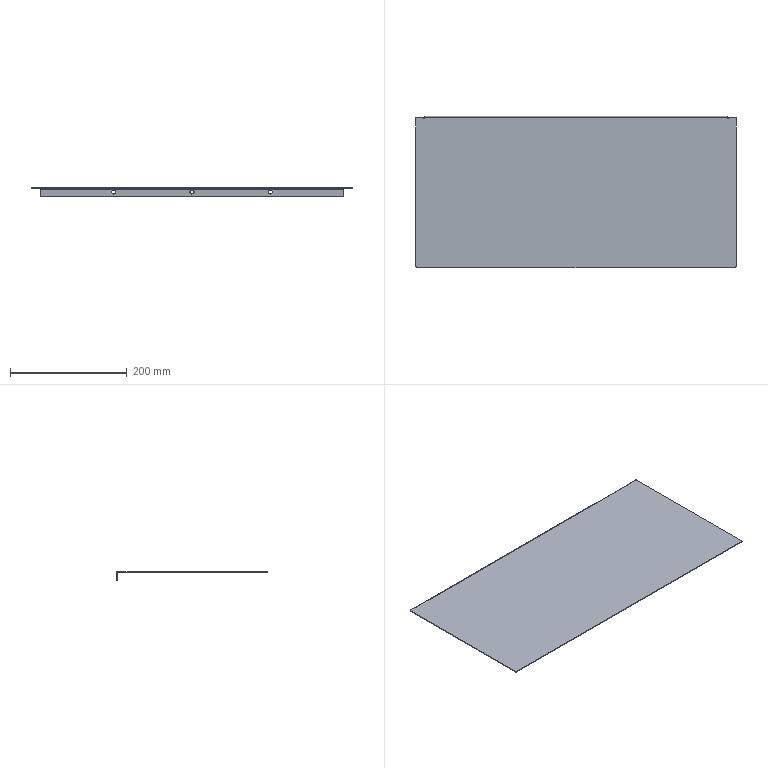Part | SolidWorks | features EdgeFlange 1, FlatPattern 1, ICE 1, SMBaseFlange 1, SheetMetal 1 | 1 solid | 32 faces | box 547.6 x 258.8 x 15 mm | volume 177930 mm3 | plane 20 | cylinder 12 | commonest cylinder face diameters 7 x6 3 x5 5.4 x1
STEP:
#1=CARTESIAN_POINT('',(133.75,258.8,-11.));
#2=VERTEX_POINT('',#1);
#3=CARTESIAN_POINT('',(133.75,258.8,-4.));
#4=VERTEX_POINT('',#3);
#5=CARTESIAN_POINT('',(133.75,258.8,-7.5));
#6=DIRECTION('',(0.,1.,0.));
#7=DIRECTION('',(0.,0.,1.));
#8=AXIS2_PLACEMENT_3D('',#5,#6,#7);
#9=CIRCLE('',#8,3.5);
#10=EDGE_CURVE('',#2,#4,#9,.T.);
#11=ORIENTED_EDGE('',*,*,#10,.F.);
#12=CARTESIAN_POINT('',(133.75,260.,-11.));
#13=VERTEX_POINT('',#12);
#14=CARTESIAN_POINT('',(133.75,250.,-11.));
#15=DIRECTION('',(0.,1.,0.));
#16=VECTOR('',#15,1000.);
#17=LINE('',#14,#16);
#18=EDGE_CURVE('',#2,#13,#17,.T.);
#19=ORIENTED_EDGE('',*,*,#18,.T.);
#20=CARTESIAN_POINT('',(133.75,260.,-4.));
#21=VERTEX_POINT('',#20);
#22=CARTESIAN_POINT('',(133.75,260.,-7.5));
#23=DIRECTION('',(0.,1.,0.));
#24=DIRECTION('',(0.,0.,1.));
#25=AXIS2_PLACEMENT_3D('',#22,#23,#24);
#26=CIRCLE('',#25,3.5);
#27=EDGE_CURVE('',#13,#21,#26,.T.);
#28=ORIENTED_EDGE('',*,*,#27,.T.);
#29=CARTESIAN_POINT('',(133.75,250.,-4.));
#30=DIRECTION('',(0.,1.,0.));
#31=VECTOR('',#30,1000.);
#32=LINE('',#29,#31);
#33=EDGE_CURVE('',#4,#21,#32,.T.);
#34=ORIENTED_EDGE('',*,*,#33,.F.);
#35=EDGE_LOOP('',(#11,#19,#28,#34));
#36=FACE_OUTER_BOUND('',#35,.T.);
#37=CARTESIAN_POINT('',(133.75,250.,-7.5));
#38=DIRECTION('',(0.,1.,0.));
#39=DIRECTION('',(0.,0.,1.));
#40=AXIS2_PLACEMENT_3D('',#37,#38,#39);
#41=CYLINDRICAL_SURFACE('',#40,3.5);
#42=ADVANCED_FACE('',(#36),#41,.F.);
#43=CARTESIAN_POINT('',(-133.75,258.8,-11.));
#44=VERTEX_POINT('',#43);
#45=CARTESIAN_POINT('',(-133.75,258.8,-4.));
#46=VERTEX_POINT('',#45);
#47=CARTESIAN_POINT('',(-133.75,258.8,-7.5));
#48=DIRECTION('',(0.,1.,0.));
#49=DIRECTION('',(0.,0.,1.));
#50=AXIS2_PLACEMENT_3D('',#47,#48,#49);
#51=CIRCLE('',#50,3.5);
#52=EDGE_CURVE('',#44,#46,#51,.T.);
#53=ORIENTED_EDGE('',*,*,#52,.F.);
#54=CARTESIAN_POINT('',(-133.75,260.,-11.));
#55=VERTEX_POINT('',#54);
#56=CARTESIAN_POINT('',(-133.75,250.,-11.));
#57=DIRECTION('',(0.,1.,0.));
#58=VECTOR('',#57,1000.);
#59=LINE('',#56,#58);
#60=EDGE_CURVE('',#44,#55,#59,.T.);
#61=ORIENTED_EDGE('',*,*,#60,.T.);
#62=CARTESIAN_POINT('',(-133.75,260.,-4.));
#63=VERTEX_POINT('',#62);
#64=CARTESIAN_POINT('',(-133.75,260.,-7.5));
#65=DIRECTION('',(0.,1.,0.));
#66=DIRECTION('',(0.,0.,1.));
#67=AXIS2_PLACEMENT_3D('',#64,#65,#66);
#68=CIRCLE('',#67,3.5);
#69=EDGE_CURVE('',#55,#63,#68,.T.);
#70=ORIENTED_EDGE('',*,*,#69,.T.);
#71=CARTESIAN_POINT('',(-133.75,250.,-4.));
#72=DIRECTION('',(0.,1.,0.));
#73=VECTOR('',#72,1000.);
#74=LINE('',#71,#73);
#75=EDGE_CURVE('',#46,#63,#74,.T.);
#76=ORIENTED_EDGE('',*,*,#75,.F.);
#77=EDGE_LOOP('',(#53,#61,#70,#76));
#78=FACE_OUTER_BOUND('',#77,.T.);
#79=CARTESIAN_POINT('',(-133.75,250.,-7.5));
#80=DIRECTION('',(0.,1.,0.));
#81=DIRECTION('',(0.,0.,1.));
#82=AXIS2_PLACEMENT_3D('',#79,#80,#81);
#83=CYLINDRICAL_SURFACE('',#82,3.5);
#84=ADVANCED_FACE('',(#78),#83,.F.);
#85=CARTESIAN_POINT('',(0.,258.8,-11.));
#86=VERTEX_POINT('',#85);
#87=CARTESIAN_POINT('',(0.,258.8,-4.));
#88=VERTEX_POINT('',#87);
#89=CARTESIAN_POINT('',(0.,258.8,-7.5));
#90=DIRECTION('',(0.,1.,0.));
#91=DIRECTION('',(0.,0.,1.));
#92=AXIS2_PLACEMENT_3D('',#89,#90,#91);
#93=CIRCLE('',#92,3.5);
#94=EDGE_CURVE('',#86,#88,#93,.T.);
#95=ORIENTED_EDGE('',*,*,#94,.F.);
#96=CARTESIAN_POINT('',(0.,260.,-11.));
#97=VERTEX_POINT('',#96);
#98=CARTESIAN_POINT('',(0.,250.,-11.));
#99=DIRECTION('',(0.,1.,0.));
#100=VECTOR('',#99,1000.);
#101=LINE('',#98,#100);
#102=EDGE_CURVE('',#86,#97,#101,.T.);
#103=ORIENTED_EDGE('',*,*,#102,.T.);
#104=CARTESIAN_POINT('',(0.,260.,-4.));
#105=VERTEX_POINT('',#104);
#106=CARTESIAN_POINT('',(0.,260.,-7.5));
#107=DIRECTION('',(0.,1.,0.));
#108=DIRECTION('',(0.,0.,1.));
#109=AXIS2_PLACEMENT_3D('',#106,#107,#108);
#110=CIRCLE('',#109,3.5);
#111=EDGE_CURVE('',#97,#105,#110,.T.);
#112=ORIENTED_EDGE('',*,*,#111,.T.);
#113=CARTESIAN_POINT('',(0.,250.,-4.));
#114=DIRECTION('',(0.,1.,0.));
#115=VECTOR('',#114,1000.);
#116=LINE('',#113,#115);
#117=EDGE_CURVE('',#88,#105,#116,.T.);
#118=ORIENTED_EDGE('',*,*,#117,.F.);
#119=EDGE_LOOP('',(#95,#103,#112,#118));
#120=FACE_OUTER_BOUND('',#119,.T.);
#121=CARTESIAN_POINT('',(0.,250.,-7.5));
#122=DIRECTION('',(0.,1.,0.));
#123=DIRECTION('',(0.,0.,1.));
#124=AXIS2_PLACEMENT_3D('',#121,#122,#123);
#125=CYLINDRICAL_SURFACE('',#124,3.5);
#126=ADVANCED_FACE('',(#120),#125,.F.);
#127=CARTESIAN_POINT('',(-260.12,258.8,0.));
#128=VERTEX_POINT('',#127);
#129=CARTESIAN_POINT('',(-272.3,258.8,0.));
#130=VERTEX_POINT('',#129);
#131=CARTESIAN_POINT('',(-272.3,258.8,0.));
#132=DIRECTION('',(-1.,0.,0.));
#133=VECTOR('',#132,1000.);
#134=LINE('',#131,#133);
#135=EDGE_CURVE('',#128,#130,#134,.T.);
#136=ORIENTED_EDGE('',*,*,#135,.F.);
#137=CARTESIAN_POINT('',(-260.12,258.8,-1.2));
#138=VERTEX_POINT('',#137);
#139=CARTESIAN_POINT('',(-260.12,258.8,-1.2));
#140=DIRECTION('',(0.,0.,-1.));
#141=VECTOR('',#140,1000.);
#142=LINE('',#139,#141);
#143=EDGE_CURVE('',#128,#138,#142,.T.);
#144=ORIENTED_EDGE('',*,*,#143,.T.);
#145=CARTESIAN_POINT('',(-272.3,258.8,-1.2));
#146=VERTEX_POINT('',#145);
#147=CARTESIAN_POINT('',(-272.3,258.8,-1.2));
#148=DIRECTION('',(-1.,0.,0.));
#149=VECTOR('',#148,1000.);
#150=LINE('',#147,#149);
#151=EDGE_CURVE('',#138,#146,#150,.T.);
#152=ORIENTED_EDGE('',*,*,#151,.T.);
#153=CARTESIAN_POINT('',(-272.3,258.8,-1.2));
#154=DIRECTION('',(0.,0.,1.));
#155=VECTOR('',#154,1000.);
#156=LINE('',#153,#155);
#157=EDGE_CURVE('',#146,#130,#156,.T.);
#158=ORIENTED_EDGE('',*,*,#157,.T.);
#159=EDGE_LOOP('',(#136,#144,#152,#158));
#160=FACE_OUTER_BOUND('',#159,.T.);
#161=CARTESIAN_POINT('',(-272.3,258.8,-1.2));
#162=DIRECTION('',(0.,1.,0.));
#163=DIRECTION('',(0.,0.,1.));
#164=AXIS2_PLACEMENT_3D('',#161,#162,#163);
#165=PLANE('',#164);
#166=ADVANCED_FACE('',(#160),#165,.T.);
#167=CARTESIAN_POINT('',(272.3,258.8,-1.2));
#168=VERTEX_POINT('',#167);
#169=CARTESIAN_POINT('',(260.12,258.8,-1.2));
#170=VERTEX_POINT('',#169);
#171=CARTESIAN_POINT('',(260.,258.8,-1.2));
#172=DIRECTION('',(-1.,0.,0.));
#173=VECTOR('',#172,1000.);
#174=LINE('',#171,#173);
#175=EDGE_CURVE('',#168,#170,#174,.T.);
#176=ORIENTED_EDGE('',*,*,#175,.T.);
#177=CARTESIAN_POINT('',(260.12,258.8,0.));
#178=VERTEX_POINT('',#177);
#179=CARTESIAN_POINT('',(260.12,258.8,-1.2));
#180=DIRECTION('',(0.,0.,1.));
#181=VECTOR('',#180,1000.);
#182=LINE('',#179,#181);
#183=EDGE_CURVE('',#170,#178,#182,.T.);
#184=ORIENTED_EDGE('',*,*,#183,.T.);
#185=CARTESIAN_POINT('',(272.3,258.8,0.));
#186=VERTEX_POINT('',#185);
#187=CARTESIAN_POINT('',(260.,258.8,0.));
#188=DIRECTION('',(-1.,0.,0.));
#189=VECTOR('',#188,1000.);
#190=LINE('',#187,#189);
#191=EDGE_CURVE('',#186,#178,#190,.T.);
#192=ORIENTED_EDGE('',*,*,#191,.F.);
#193=CARTESIAN_POINT('',(272.3,258.8,-1.2));
#194=DIRECTION('',(0.,0.,1.));
#195=VECTOR('',#194,1000.);
#196=LINE('',#193,#195);
#197=EDGE_CURVE('',#168,#186,#196,.T.);
#198=ORIENTED_EDGE('',*,*,#197,.F.);
#199=EDGE_LOOP('',(#176,#184,#192,#198));
#200=FACE_OUTER_BOUND('',#199,.T.);
#201=CARTESIAN_POINT('',(260.,258.8,-1.2));
#202=DIRECTION('',(0.,1.,0.));
#203=DIRECTION('',(0.,0.,1.));
#204=AXIS2_PLACEMENT_3D('',#201,#202,#203);
#205=PLANE('',#204);
#206=ADVANCED_FACE('',(#200),#205,.T.);
#207=CARTESIAN_POINT('',(260.12,257.18,-1.2));
#208=VERTEX_POINT('',#207);
#209=CARTESIAN_POINT('',(260.12,260.,-1.2));
#210=DIRECTION('',(0.,-1.,0.));
#211=VECTOR('',#210,1000.);
#212=LINE('',#209,#211);
#213=EDGE_CURVE('',#170,#208,#212,.T.);
#214=ORIENTED_EDGE('',*,*,#213,.F.);
#215=ORIENTED_EDGE('',*,*,#175,.F.);
#216=CARTESIAN_POINT('',(273.8,257.3,-1.2));
#217=VERTEX_POINT('',#216);
#218=CARTESIAN_POINT('',(272.3,257.3,-1.2));
#219=DIRECTION('',(0.,0.,1.));
#220=DIRECTION('',(1.,0.,0.));
#221=AXIS2_PLACEMENT_3D('',#218,#219,#220);
#222=CIRCLE('',#221,1.5);
#223=EDGE_CURVE('',#217,#168,#222,.T.);
#224=ORIENTED_EDGE('',*,*,#223,.F.);
#225=CARTESIAN_POINT('',(273.8,2.7,-1.2));
#226=VERTEX_POINT('',#225);
#227=CARTESIAN_POINT('',(273.8,257.3,-1.2));
#228=DIRECTION('',(0.,1.,0.));
#229=VECTOR('',#228,1000.);
#230=LINE('',#227,#229);
#231=EDGE_CURVE('',#226,#217,#230,.T.);
#232=ORIENTED_EDGE('',*,*,#231,.F.);
#233=CARTESIAN_POINT('',(272.3,1.2,-1.2));
#234=VERTEX_POINT('',#233);
#235=CARTESIAN_POINT('',(272.3,2.7,-1.2));
#236=DIRECTION('',(0.,0.,1.));
#237=DIRECTION('',(1.,0.,0.));
#238=AXIS2_PLACEMENT_3D('',#235,#236,#237);
#239=CIRCLE('',#238,1.5);
#240=EDGE_CURVE('',#234,#226,#239,.T.);
#241=ORIENTED_EDGE('',*,*,#240,.F.);
#242=CARTESIAN_POINT('',(-272.3,1.2,-1.2));
#243=VERTEX_POINT('',#242);
#244=CARTESIAN_POINT('',(272.3,1.2,-1.2));
#245=DIRECTION('',(1.,0.,0.));
#246=VECTOR('',#245,1000.);
#247=LINE('',#244,#246);
#248=EDGE_CURVE('',#243,#234,#247,.T.);
#249=ORIENTED_EDGE('',*,*,#248,.F.);
#250=CARTESIAN_POINT('',(-273.8,2.7,-1.2));
#251=VERTEX_POINT('',#250);
#252=CARTESIAN_POINT('',(-272.3,2.7,-1.2));
#253=DIRECTION('',(0.,0.,1.));
#254=DIRECTION('',(1.,0.,0.));
#255=AXIS2_PLACEMENT_3D('',#252,#253,#254);
#256=CIRCLE('',#255,1.5);
#257=EDGE_CURVE('',#251,#243,#256,.T.);
#258=ORIENTED_EDGE('',*,*,#257,.F.);
#259=CARTESIAN_POINT('',(-273.8,257.3,-1.2));
#260=VERTEX_POINT('',#259);
#261=CARTESIAN_POINT('',(-273.8,2.7,-1.2));
#262=DIRECTION('',(0.,-1.,0.));
#263=VECTOR('',#262,1000.);
#264=LINE('',#261,#263);
#265=EDGE_CURVE('',#260,#251,#264,.T.);
#266=ORIENTED_EDGE('',*,*,#265,.F.);
#267=CARTESIAN_POINT('',(-272.3,257.3,-1.2));
#268=DIRECTION('',(0.,0.,1.));
#269=DIRECTION('',(1.,0.,0.));
#270=AXIS2_PLACEMENT_3D('',#267,#268,#269);
#271=CIRCLE('',#270,1.5);
#272=EDGE_CURVE('',#146,#260,#271,.T.);
#273=ORIENTED_EDGE('',*,*,#272,.F.);
#274=ORIENTED_EDGE('',*,*,#151,.F.);
#275=CARTESIAN_POINT('',(-260.12,257.18,-1.2));
#276=VERTEX_POINT('',#275);
#277=CARTESIAN_POINT('',(-260.12,257.18,-1.2));
#278=DIRECTION('',(0.,1.,0.));
#279=VECTOR('',#278,1000.);
#280=LINE('',#277,#279);
#281=EDGE_CURVE('',#276,#138,#280,.T.);
#282=ORIENTED_EDGE('',*,*,#281,.F.);
#283=CARTESIAN_POINT('',(-260.,257.18,-1.2));
#284=VERTEX_POINT('',#283);
#285=CARTESIAN_POINT('',(-260.,257.18,-1.2));
#286=DIRECTION('',(-1.,0.,0.));
#287=VECTOR('',#286,1000.);
#288=LINE('',#285,#287);
#289=EDGE_CURVE('',#284,#276,#288,.T.);
#290=ORIENTED_EDGE('',*,*,#289,.F.);
#291=CARTESIAN_POINT('',(-260.,257.3,-1.2));
#292=VERTEX_POINT('',#291);
#293=CARTESIAN_POINT('',(-260.,257.3,-1.2));
#294=DIRECTION('',(0.,-1.,0.));
#295=VECTOR('',#294,1000.);
#296=LINE('',#293,#295);
#297=EDGE_CURVE('',#292,#284,#296,.T.);
#298=ORIENTED_EDGE('',*,*,#297,.F.);
#299=CARTESIAN_POINT('',(260.,257.3,-1.2));
#300=VERTEX_POINT('',#299);
#301=CARTESIAN_POINT('',(260.,257.3,-1.2));
#302=DIRECTION('',(-1.,0.,0.));
#303=VECTOR('',#302,1000.);
#304=LINE('',#301,#303);
#305=EDGE_CURVE('',#300,#292,#304,.T.);
#306=ORIENTED_EDGE('',*,*,#305,.F.);
#307=CARTESIAN_POINT('',(260.,257.18,-1.2));
#308=VERTEX_POINT('',#307);
#309=CARTESIAN_POINT('',(260.,257.18,-1.2));
#310=DIRECTION('',(0.,1.,0.));
#311=VECTOR('',#310,1000.);
#312=LINE('',#309,#311);
#313=EDGE_CURVE('',#308,#300,#312,.T.);
#314=ORIENTED_EDGE('',*,*,#313,.F.);
#315=CARTESIAN_POINT('',(260.12,257.18,-1.2));
#316=DIRECTION('',(-1.,0.,0.));
#317=VECTOR('',#316,1000.);
#318=LINE('',#315,#317);
#319=EDGE_CURVE('',#208,#308,#318,.T.);
#320=ORIENTED_EDGE('',*,*,#319,.F.);
#321=EDGE_LOOP('',(#214,#215,#224,#232,#241,#249,#258,#266,#273,#274,#282,#290,#298,#306,#314,#320));
#322=FACE_OUTER_BOUND('',#321,.T.);
#323=CARTESIAN_POINT('',(-272.3,257.3,-1.2));
#324=DIRECTION('',(0.,0.,1.));
#325=DIRECTION('',(1.,0.,0.));
#326=AXIS2_PLACEMENT_3D('',#323,#324,#325);
#327=PLANE('',#326);
#328=ADVANCED_FACE('',(#322),#327,.F.);
#329=ORIENTED_EDGE('',*,*,#191,.T.);
#330=CARTESIAN_POINT('',(260.12,257.18,0.));
#331=VERTEX_POINT('',#330);
#332=CARTESIAN_POINT('',(260.12,257.3,0.));
#333=DIRECTION('',(0.,-1.,0.));
#334=VECTOR('',#333,1000.);
#335=LINE('',#332,#334);
#336=EDGE_CURVE('',#178,#331,#335,.T.);
#337=ORIENTED_EDGE('',*,*,#336,.T.);
#338=CARTESIAN_POINT('',(260.,257.18,0.));
#339=VERTEX_POINT('',#338);
#340=CARTESIAN_POINT('',(-272.3,257.18,0.));
#341=DIRECTION('',(-1.,0.,0.));
#342=VECTOR('',#341,1000.);
#343=LINE('',#340,#342);
#344=EDGE_CURVE('',#331,#339,#343,.T.);
#345=ORIENTED_EDGE('',*,*,#344,.T.);
#346=CARTESIAN_POINT('',(260.,257.3,0.));
#347=VERTEX_POINT('',#346);
#348=CARTESIAN_POINT('',(260.,257.3,0.));
#349=DIRECTION('',(0.,1.,0.));
#350=VECTOR('',#349,1000.);
#351=LINE('',#348,#350);
#352=EDGE_CURVE('',#339,#347,#351,.T.);
#353=ORIENTED_EDGE('',*,*,#352,.T.);
#354=CARTESIAN_POINT('',(-260.,257.3,0.));
#355=VERTEX_POINT('',#354);
#356=CARTESIAN_POINT('',(260.,257.3,0.));
#357=DIRECTION('',(-1.,0.,0.));
#358=VECTOR('',#357,1000.);
#359=LINE('',#356,#358);
#360=EDGE_CURVE('',#347,#355,#359,.T.);
#361=ORIENTED_EDGE('',*,*,#360,.T.);
#362=CARTESIAN_POINT('',(-260.,257.18,0.));
#363=VERTEX_POINT('',#362);
#364=CARTESIAN_POINT('',(-260.,257.3,0.));
#365=DIRECTION('',(0.,-1.,0.));
#366=VECTOR('',#365,1000.);
#367=LINE('',#364,#366);
#368=EDGE_CURVE('',#355,#363,#367,.T.);
#369=ORIENTED_EDGE('',*,*,#368,.T.);
#370=CARTESIAN_POINT('',(-260.12,257.18,0.));
#371=VERTEX_POINT('',#370);
#372=CARTESIAN_POINT('',(-272.3,257.18,0.));
#373=DIRECTION('',(-1.,0.,0.));
#374=VECTOR('',#373,1000.);
#375=LINE('',#372,#374);
#376=EDGE_CURVE('',#363,#371,#375,.T.);
#377=ORIENTED_EDGE('',*,*,#376,.T.);
#378=CARTESIAN_POINT('',(-260.12,257.3,0.));
#379=DIRECTION('',(0.,1.,0.));
#380=VECTOR('',#379,1000.);
#381=LINE('',#378,#380);
#382=EDGE_CURVE('',#371,#128,#381,.T.);
#383=ORIENTED_EDGE('',*,*,#382,.T.);
#384=ORIENTED_EDGE('',*,*,#135,.T.);
#385=CARTESIAN_POINT('',(-273.8,257.3,0.));
#386=VERTEX_POINT('',#385);
#387=CARTESIAN_POINT('',(-272.3,257.3,0.));
#388=DIRECTION('',(0.,0.,1.));
#389=DIRECTION('',(1.,0.,0.));
#390=AXIS2_PLACEMENT_3D('',#387,#388,#389);
#391=CIRCLE('',#390,1.5);
#392=EDGE_CURVE('',#130,#386,#391,.T.);
#393=ORIENTED_EDGE('',*,*,#392,.T.);
#394=CARTESIAN_POINT('',(-273.8,2.7,0.));
#395=VERTEX_POINT('',#394);
#396=CARTESIAN_POINT('',(-273.8,2.7,0.));
#397=DIRECTION('',(0.,-1.,0.));
#398=VECTOR('',#397,1000.);
#399=LINE('',#396,#398);
#400=EDGE_CURVE('',#386,#395,#399,.T.);
#401=ORIENTED_EDGE('',*,*,#400,.T.);
#402=CARTESIAN_POINT('',(-272.3,1.2,0.));
#403=VERTEX_POINT('',#402);
#404=CARTESIAN_POINT('',(-272.3,2.7,0.));
#405=DIRECTION('',(0.,0.,1.));
#406=DIRECTION('',(1.,0.,0.));
#407=AXIS2_PLACEMENT_3D('',#404,#405,#406);
#408=CIRCLE('',#407,1.5);
#409=EDGE_CURVE('',#395,#403,#408,.T.);
#410=ORIENTED_EDGE('',*,*,#409,.T.);
#411=CARTESIAN_POINT('',(272.3,1.2,0.));
#412=VERTEX_POINT('',#411);
#413=CARTESIAN_POINT('',(272.3,1.2,0.));
#414=DIRECTION('',(1.,0.,0.));
#415=VECTOR('',#414,1000.);
#416=LINE('',#413,#415);
#417=EDGE_CURVE('',#403,#412,#416,.T.);
#418=ORIENTED_EDGE('',*,*,#417,.T.);
#419=CARTESIAN_POINT('',(273.8,2.7,0.));
#420=VERTEX_POINT('',#419);
#421=CARTESIAN_POINT('',(272.3,2.7,0.));
#422=DIRECTION('',(0.,0.,1.));
#423=DIRECTION('',(1.,0.,0.));
#424=AXIS2_PLACEMENT_3D('',#421,#422,#423);
#425=CIRCLE('',#424,1.5);
#426=EDGE_CURVE('',#412,#420,#425,.T.);
#427=ORIENTED_EDGE('',*,*,#426,.T.);
#428=CARTESIAN_POINT('',(273.8,257.3,0.));
#429=VERTEX_POINT('',#428);
#430=CARTESIAN_POINT('',(273.8,257.3,0.));
#431=DIRECTION('',(0.,1.,0.));
#432=VECTOR('',#431,1000.);
#433=LINE('',#430,#432);
#434=EDGE_CURVE('',#420,#429,#433,.T.);
#435=ORIENTED_EDGE('',*,*,#434,.T.);
#436=CARTESIAN_POINT('',(272.3,257.3,0.));
#437=DIRECTION('',(0.,0.,1.));
#438=DIRECTION('',(1.,0.,0.));
#439=AXIS2_PLACEMENT_3D('',#436,#437,#438);
#440=CIRCLE('',#439,1.5);
#441=EDGE_CURVE('',#429,#186,#440,.T.);
#442=ORIENTED_EDGE('',*,*,#441,.T.);
#443=EDGE_LOOP('',(#329,#337,#345,#353,#361,#369,#377,#383,#384,#393,#401,#410,#418,#427,#435,#442));
#444=FACE_OUTER_BOUND('',#443,.T.);
#445=CARTESIAN_POINT('',(-272.3,257.3,0.));
#446=DIRECTION('',(0.,0.,1.));
#447=DIRECTION('',(1.,0.,0.));
#448=AXIS2_PLACEMENT_3D('',#445,#446,#447);
#449=PLANE('',#448);
#450=ADVANCED_FACE('',(#444),#449,.T.);
#451=ORIENTED_EDGE('',*,*,#392,.F.);
#452=ORIENTED_EDGE('',*,*,#157,.F.);
#453=ORIENTED_EDGE('',*,*,#272,.T.);
#454=CARTESIAN_POINT('',(-273.8,257.3,-1.2));
#455=DIRECTION('',(0.,0.,1.));
#456=VECTOR('',#455,1000.);
#457=LINE('',#454,#456);
#458=EDGE_CURVE('',#260,#386,#457,.T.);
#459=ORIENTED_EDGE('',*,*,#458,.T.);
#460=EDGE_LOOP('',(#451,#452,#453,#459));
#461=FACE_OUTER_BOUND('',#460,.T.);
#462=CARTESIAN_POINT('',(-272.3,257.3,-1.2));
#463=DIRECTION('',(0.,0.,1.));
#464=DIRECTION('',(1.,0.,0.));
#465=AXIS2_PLACEMENT_3D('',#462,#463,#464);
#466=CYLINDRICAL_SURFACE('',#465,1.5);
#467=ADVANCED_FACE('',(#461),#466,.T.);
#468=ORIENTED_EDGE('',*,*,#441,.F.);
#469=CARTESIAN_POINT('',(273.8,257.3,-1.2));
#470=DIRECTION('',(0.,0.,1.));
#471=VECTOR('',#470,1000.);
#472=LINE('',#469,#471);
#473=EDGE_CURVE('',#217,#429,#472,.T.);
#474=ORIENTED_EDGE('',*,*,#473,.F.);
#475=ORIENTED_EDGE('',*,*,#223,.T.);
#476=ORIENTED_EDGE('',*,*,#197,.T.);
#477=EDGE_LOOP('',(#468,#474,#475,#476));
#478=FACE_OUTER_BOUND('',#477,.T.);
#479=CARTESIAN_POINT('',(272.3,257.3,-1.2));
#480=DIRECTION('',(0.,0.,1.));
#481=DIRECTION('',(1.,0.,0.));
#482=AXIS2_PLACEMENT_3D('',#479,#480,#481);
#483=CYLINDRICAL_SURFACE('',#482,1.5);
#484=ADVANCED_FACE('',(#478),#483,.T.);
#485=ORIENTED_EDGE('',*,*,#434,.F.);
#486=CARTESIAN_POINT('',(273.8,2.7,-1.2));
#487=DIRECTION('',(0.,0.,1.));
#488=VECTOR('',#487,1000.);
#489=LINE('',#486,#488);
#490=EDGE_CURVE('',#226,#420,#489,.T.);
#491=ORIENTED_EDGE('',*,*,#490,.F.);
#492=ORIENTED_EDGE('',*,*,#231,.T.);
#493=ORIENTED_EDGE('',*,*,#473,.T.);
#494=EDGE_LOOP('',(#485,#491,#492,#493));
#495=FACE_OUTER_BOUND('',#494,.T.);
#496=CARTESIAN_POINT('',(273.8,257.3,-1.2));
#497=DIRECTION('',(1.,0.,0.));
#498=DIRECTION('',(0.,1.,0.));
#499=AXIS2_PLACEMENT_3D('',#496,#497,#498);
#500=PLANE('',#499);
#501=ADVANCED_FACE('',(#495),#500,.T.);
#502=ORIENTED_EDGE('',*,*,#426,.F.);
#503=CARTESIAN_POINT('',(272.3,1.2,-1.2));
#504=DIRECTION('',(0.,0.,1.));
#505=VECTOR('',#504,1000.);
#506=LINE('',#503,#505);
#507=EDGE_CURVE('',#234,#412,#506,.T.);
#508=ORIENTED_EDGE('',*,*,#507,.F.);
#509=ORIENTED_EDGE('',*,*,#240,.T.);
#510=ORIENTED_EDGE('',*,*,#490,.T.);
#511=EDGE_LOOP('',(#502,#508,#509,#510));
#512=FACE_OUTER_BOUND('',#511,.T.);
#513=CARTESIAN_POINT('',(272.3,2.7,-1.2));
#514=DIRECTION('',(0.,0.,1.));
#515=DIRECTION('',(1.,0.,0.));
#516=AXIS2_PLACEMENT_3D('',#513,#514,#515);
#517=CYLINDRICAL_SURFACE('',#516,1.5);
#518=ADVANCED_FACE('',(#512),#517,.T.);
#519=ORIENTED_EDGE('',*,*,#417,.F.);
#520=CARTESIAN_POINT('',(-272.3,1.2,-1.2));
#521=DIRECTION('',(0.,0.,1.));
#522=VECTOR('',#521,1000.);
#523=LINE('',#520,#522);
#524=EDGE_CURVE('',#243,#403,#523,.T.);
#525=ORIENTED_EDGE('',*,*,#524,.F.);
#526=ORIENTED_EDGE('',*,*,#248,.T.);
#527=ORIENTED_EDGE('',*,*,#507,.T.);
#528=EDGE_LOOP('',(#519,#525,#526,#527));
#529=FACE_OUTER_BOUND('',#528,.T.);
#530=CARTESIAN_POINT('',(272.3,1.2,-1.2));
#531=DIRECTION('',(0.,-1.,0.));
#532=DIRECTION('',(0.,0.,-1.));
#533=AXIS2_PLACEMENT_3D('',#530,#531,#532);
#534=PLANE('',#533);
#535=ADVANCED_FACE('',(#529),#534,.T.);
#536=ORIENTED_EDGE('',*,*,#409,.F.);
#537=CARTESIAN_POINT('',(-273.8,2.7,-1.2));
#538=DIRECTION('',(0.,0.,1.));
#539=VECTOR('',#538,1000.);
#540=LINE('',#537,#539);
#541=EDGE_CURVE('',#251,#395,#540,.T.);
#542=ORIENTED_EDGE('',*,*,#541,.F.);
#543=ORIENTED_EDGE('',*,*,#257,.T.);
#544=ORIENTED_EDGE('',*,*,#524,.T.);
#545=EDGE_LOOP('',(#536,#542,#543,#544));
#546=FACE_OUTER_BOUND('',#545,.T.);
#547=CARTESIAN_POINT('',(-272.3,2.7,-1.2));
#548=DIRECTION('',(0.,0.,1.));
#549=DIRECTION('',(1.,0.,0.));
#550=AXIS2_PLACEMENT_3D('',#547,#548,#549);
#551=CYLINDRICAL_SURFACE('',#550,1.5);
#552=ADVANCED_FACE('',(#546),#551,.T.);
#553=ORIENTED_EDGE('',*,*,#400,.F.);
#554=ORIENTED_EDGE('',*,*,#458,.F.);
#555=ORIENTED_EDGE('',*,*,#265,.T.);
#556=ORIENTED_EDGE('',*,*,#541,.T.);
#557=EDGE_LOOP('',(#553,#554,#555,#556));
#558=FACE_OUTER_BOUND('',#557,.T.);
#559=CARTESIAN_POINT('',(-273.8,2.7,-1.2));
#560=DIRECTION('',(-1.,0.,0.));
#561=DIRECTION('',(0.,0.,1.));
#562=AXIS2_PLACEMENT_3D('',#559,#560,#561);
#563=PLANE('',#562);
#564=ADVANCED_FACE('',(#558),#563,.T.);
#565=ORIENTED_EDGE('',*,*,#183,.F.);
#566=ORIENTED_EDGE('',*,*,#213,.T.);
#567=CARTESIAN_POINT('',(260.12,257.18,-1.2));
#568=DIRECTION('',(0.,0.,1.));
#569=VECTOR('',#568,1000.);
#570=LINE('',#567,#569);
#571=EDGE_CURVE('',#208,#331,#570,.T.);
#572=ORIENTED_EDGE('',*,*,#571,.T.);
#573=ORIENTED_EDGE('',*,*,#336,.F.);
#574=EDGE_LOOP('',(#565,#566,#572,#573));
#575=FACE_OUTER_BOUND('',#574,.T.);
#576=CARTESIAN_POINT('',(260.12,260.,-1.2));
#577=DIRECTION('',(-1.,0.,0.));
#578=DIRECTION('',(0.,0.,1.));
#579=AXIS2_PLACEMENT_3D('',#576,#577,#578);
#580=PLANE('',#579);
#581=ADVANCED_FACE('',(#575),#580,.T.);
#582=ORIENTED_EDGE('',*,*,#344,.F.);
#583=ORIENTED_EDGE('',*,*,#571,.F.);
#584=ORIENTED_EDGE('',*,*,#319,.T.);
#585=CARTESIAN_POINT('',(260.,257.18,-1.2));
#586=DIRECTION('',(0.,0.,1.));
#587=VECTOR('',#586,1000.);
#588=LINE('',#585,#587);
#589=EDGE_CURVE('',#308,#339,#588,.T.);
#590=ORIENTED_EDGE('',*,*,#589,.T.);
#591=EDGE_LOOP('',(#582,#583,#584,#590));
#592=FACE_OUTER_BOUND('',#591,.T.);
#593=CARTESIAN_POINT('',(260.12,257.18,-1.2));
#594=DIRECTION('',(0.,1.,0.));
#595=DIRECTION('',(0.,0.,1.));
#596=AXIS2_PLACEMENT_3D('',#593,#594,#595);
#597=PLANE('',#596);
#598=ADVANCED_FACE('',(#592),#597,.T.);
#599=ORIENTED_EDGE('',*,*,#352,.F.);
#600=ORIENTED_EDGE('',*,*,#589,.F.);
#601=ORIENTED_EDGE('',*,*,#313,.T.);
#602=CARTESIAN_POINT('',(260.,257.3,-1.2));
#603=DIRECTION('',(0.,0.,1.));
#604=VECTOR('',#603,1000.);
#605=LINE('',#602,#604);
#606=EDGE_CURVE('',#300,#347,#605,.T.);
#607=ORIENTED_EDGE('',*,*,#606,.T.);
#608=EDGE_LOOP('',(#599,#600,#601,#607));
#609=FACE_OUTER_BOUND('',#608,.T.);
#610=CARTESIAN_POINT('',(260.,257.18,-1.2));
#611=DIRECTION('',(1.,0.,0.));
#612=DIRECTION('',(0.,0.,-1.));
#613=AXIS2_PLACEMENT_3D('',#610,#611,#612);
#614=PLANE('',#613);
#615=ADVANCED_FACE('',(#609),#614,.T.);
#616=ORIENTED_EDGE('',*,*,#368,.F.);
#617=CARTESIAN_POINT('',(-260.,257.3,-1.2));
#618=DIRECTION('',(0.,0.,1.));
#619=VECTOR('',#618,1000.);
#620=LINE('',#617,#619);
#621=EDGE_CURVE('',#292,#355,#620,.T.);
#622=ORIENTED_EDGE('',*,*,#621,.F.);
#623=ORIENTED_EDGE('',*,*,#297,.T.);
#624=CARTESIAN_POINT('',(-260.,257.18,-1.2));
#625=DIRECTION('',(0.,0.,1.));
#626=VECTOR('',#625,1000.);
#627=LINE('',#624,#626);
#628=EDGE_CURVE('',#284,#363,#627,.T.);
#629=ORIENTED_EDGE('',*,*,#628,.T.);
#630=EDGE_LOOP('',(#616,#622,#623,#629));
#631=FACE_OUTER_BOUND('',#630,.T.);
#632=CARTESIAN_POINT('',(-260.,257.3,-1.2));
#633=DIRECTION('',(-1.,0.,0.));
#634=DIRECTION('',(0.,0.,1.));
#635=AXIS2_PLACEMENT_3D('',#632,#633,#634);
#636=PLANE('',#635);
#637=ADVANCED_FACE('',(#631),#636,.T.);
#638=ORIENTED_EDGE('',*,*,#376,.F.);
#639=ORIENTED_EDGE('',*,*,#628,.F.);
#640=ORIENTED_EDGE('',*,*,#289,.T.);
#641=CARTESIAN_POINT('',(-260.12,257.18,-1.2));
#642=DIRECTION('',(0.,0.,1.));
#643=VECTOR('',#642,1000.);
#644=LINE('',#641,#643);
#645=EDGE_CURVE('',#276,#371,#644,.T.);
#646=ORIENTED_EDGE('',*,*,#645,.T.);
#647=EDGE_LOOP('',(#638,#639,#640,#646));
#648=FACE_OUTER_BOUND('',#647,.T.);
#649=CARTESIAN_POINT('',(-260.,257.18,-1.2));
#650=DIRECTION('',(0.,1.,0.));
#651=DIRECTION('',(0.,0.,1.));
#652=AXIS2_PLACEMENT_3D('',#649,#650,#651);
#653=PLANE('',#652);
#654=ADVANCED_FACE('',(#648),#653,.T.);
#655=ORIENTED_EDGE('',*,*,#143,.F.);
#656=ORIENTED_EDGE('',*,*,#382,.F.);
#657=ORIENTED_EDGE('',*,*,#645,.F.);
#658=ORIENTED_EDGE('',*,*,#281,.T.);
#659=EDGE_LOOP('',(#655,#656,#657,#658));
#660=FACE_OUTER_BOUND('',#659,.T.);
#661=CARTESIAN_POINT('',(-260.12,257.18,-1.2));
#662=DIRECTION('',(1.,0.,0.));
#663=DIRECTION('',(0.,0.,-1.));
#664=AXIS2_PLACEMENT_3D('',#661,#662,#663);
#665=PLANE('',#664);
#666=ADVANCED_FACE('',(#660),#665,.T.);
#667=CARTESIAN_POINT('',(-260.,258.8,-2.7));
#668=VERTEX_POINT('',#667);
#669=CARTESIAN_POINT('',(-260.,260.,-2.7));
#670=VERTEX_POINT('',#669);
#671=CARTESIAN_POINT('',(-260.,260.,-2.7));
#672=DIRECTION('',(0.,1.,0.));
#673=VECTOR('',#672,1000.);
#674=LINE('',#671,#673);
#675=EDGE_CURVE('',#668,#670,#674,.T.);
#676=ORIENTED_EDGE('',*,*,#675,.F.);
#677=CARTESIAN_POINT('',(-260.,257.3,-2.7));
#678=DIRECTION('',(-1.,0.,0.));
#679=DIRECTION('',(0.,0.,-1.));
#680=AXIS2_PLACEMENT_3D('',#677,#678,#679);
#681=CIRCLE('',#680,1.5);
#682=EDGE_CURVE('',#292,#668,#681,.T.);
#683=ORIENTED_EDGE('',*,*,#682,.F.);
#684=ORIENTED_EDGE('',*,*,#621,.T.);
#685=CARTESIAN_POINT('',(-260.,257.3,-2.7));
#686=DIRECTION('',(-1.,0.,0.));
#687=DIRECTION('',(0.,0.,-1.));
#688=AXIS2_PLACEMENT_3D('',#685,#686,#687);
#689=CIRCLE('',#688,2.7);
#690=EDGE_CURVE('',#355,#670,#689,.T.);
#691=ORIENTED_EDGE('',*,*,#690,.T.);
#692=EDGE_LOOP('',(#676,#683,#684,#691));
#693=FACE_OUTER_BOUND('',#692,.T.);
#694=CARTESIAN_POINT('',(-260.,257.3,-2.7));
#695=DIRECTION('',(-1.,0.,0.));
#696=DIRECTION('',(0.,0.,1.));
#697=AXIS2_PLACEMENT_3D('',#694,#695,#696);
#698=PLANE('',#697);
#699=ADVANCED_FACE('',(#693),#698,.T.);
#700=CARTESIAN_POINT('',(260.,258.8,-2.7));
#701=VERTEX_POINT('',#700);
#702=CARTESIAN_POINT('',(260.,257.3,-2.7));
#703=DIRECTION('',(1.,0.,0.));
#704=DIRECTION('',(0.,0.,-1.));
#705=AXIS2_PLACEMENT_3D('',#702,#703,#704);
#706=CIRCLE('',#705,1.5);
#707=EDGE_CURVE('',#701,#300,#706,.T.);
#708=ORIENTED_EDGE('',*,*,#707,.F.);
#709=CARTESIAN_POINT('',(260.,260.,-2.7));
#710=VERTEX_POINT('',#709);
#711=CARTESIAN_POINT('',(260.,258.8,-2.7));
#712=DIRECTION('',(0.,1.,0.));
#713=VECTOR('',#712,1000.);
#714=LINE('',#711,#713);
#715=EDGE_CURVE('',#701,#710,#714,.T.);
#716=ORIENTED_EDGE('',*,*,#715,.T.);
#717=CARTESIAN_POINT('',(260.,257.3,-2.7));
#718=DIRECTION('',(1.,0.,0.));
#719=DIRECTION('',(0.,0.,-1.));
#720=AXIS2_PLACEMENT_3D('',#717,#718,#719);
#721=CIRCLE('',#720,2.7);
#722=EDGE_CURVE('',#710,#347,#721,.T.);
#723=ORIENTED_EDGE('',*,*,#722,.T.);
#724=ORIENTED_EDGE('',*,*,#606,.F.);
#725=EDGE_LOOP('',(#708,#716,#723,#724));
#726=FACE_OUTER_BOUND('',#725,.T.);
#727=CARTESIAN_POINT('',(260.,257.3,-2.7));
#728=DIRECTION('',(-1.,0.,0.));
#729=DIRECTION('',(0.,0.,1.));
#730=AXIS2_PLACEMENT_3D('',#727,#728,#729);
#731=PLANE('',#730);
#732=ADVANCED_FACE('',(#726),#731,.F.);
#733=ORIENTED_EDGE('',*,*,#360,.F.);
#734=ORIENTED_EDGE('',*,*,#722,.F.);
#735=CARTESIAN_POINT('',(0.,260.,-2.7));
#736=DIRECTION('',(1.,0.,0.));
#737=VECTOR('',#736,1000.);
#738=LINE('',#735,#737);
#739=EDGE_CURVE('',#670,#710,#738,.T.);
#740=ORIENTED_EDGE('',*,*,#739,.F.);
#741=ORIENTED_EDGE('',*,*,#690,.F.);
#742=EDGE_LOOP('',(#733,#734,#740,#741));
#743=FACE_OUTER_BOUND('',#742,.T.);
#744=CARTESIAN_POINT('',(260.,257.3,-2.7));
#745=DIRECTION('',(1.,0.,0.));
#746=DIRECTION('',(0.,1.,0.));
#747=AXIS2_PLACEMENT_3D('',#744,#745,#746);
#748=CYLINDRICAL_SURFACE('',#747,2.7);
#749=ADVANCED_FACE('',(#743),#748,.T.);
#750=ORIENTED_EDGE('',*,*,#305,.T.);
#751=ORIENTED_EDGE('',*,*,#682,.T.);
#752=CARTESIAN_POINT('',(-260.,258.8,-2.7));
#753=DIRECTION('',(1.,0.,0.));
#754=VECTOR('',#753,1000.);
#755=LINE('',#752,#754);
#756=EDGE_CURVE('',#668,#701,#755,.T.);
#757=ORIENTED_EDGE('',*,*,#756,.T.);
#758=ORIENTED_EDGE('',*,*,#707,.T.);
#759=EDGE_LOOP('',(#750,#751,#757,#758));
#760=FACE_OUTER_BOUND('',#759,.T.);
#761=CARTESIAN_POINT('',(260.,257.3,-2.7));
#762=DIRECTION('',(1.,0.,0.));
#763=DIRECTION('',(0.,1.,0.));
#764=AXIS2_PLACEMENT_3D('',#761,#762,#763);
#765=CYLINDRICAL_SURFACE('',#764,1.5);
#766=ADVANCED_FACE('',(#760),#765,.F.);
#767=CARTESIAN_POINT('',(260.,260.,-15.));
#768=VERTEX_POINT('',#767);
#769=CARTESIAN_POINT('',(260.,260.,-1.2));
#770=DIRECTION('',(0.,0.,1.));
#771=VECTOR('',#770,1000.);
#772=LINE('',#769,#771);
#773=EDGE_CURVE('',#768,#710,#772,.T.);
#774=ORIENTED_EDGE('',*,*,#773,.T.);
#775=ORIENTED_EDGE('',*,*,#715,.F.);
#776=CARTESIAN_POINT('',(260.,258.8,-15.));
#777=VERTEX_POINT('',#776);
#778=CARTESIAN_POINT('',(260.,258.8,0.));
#779=DIRECTION('',(0.,0.,1.));
#780=VECTOR('',#779,1000.);
#781=LINE('',#778,#780);
#782=EDGE_CURVE('',#777,#701,#781,.T.);
#783=ORIENTED_EDGE('',*,*,#782,.F.);
#784=CARTESIAN_POINT('',(260.,260.,-15.));
#785=DIRECTION('',(0.,-1.,0.));
#786=VECTOR('',#785,1000.);
#787=LINE('',#784,#786);
#788=EDGE_CURVE('',#768,#777,#787,.T.);
#789=ORIENTED_EDGE('',*,*,#788,.F.);
#790=EDGE_LOOP('',(#774,#775,#783,#789));
#791=FACE_OUTER_BOUND('',#790,.T.);
#792=CARTESIAN_POINT('',(260.,260.,-1.2));
#793=DIRECTION('',(1.,0.,0.));
#794=DIRECTION('',(0.,0.,-1.));
#795=AXIS2_PLACEMENT_3D('',#792,#793,#794);
#796=PLANE('',#795);
#797=ADVANCED_FACE('',(#791),#796,.T.);
#798=CARTESIAN_POINT('',(-260.,258.8,-15.));
#799=VERTEX_POINT('',#798);
#800=CARTESIAN_POINT('',(-260.,258.8,0.));
#801=DIRECTION('',(0.,0.,-1.));
#802=VECTOR('',#801,1000.);
#803=LINE('',#800,#802);
#804=EDGE_CURVE('',#668,#799,#803,.T.);
#805=ORIENTED_EDGE('',*,*,#804,.F.);
#806=ORIENTED_EDGE('',*,*,#675,.T.);
#807=CARTESIAN_POINT('',(-260.,260.,-15.));
#808=VERTEX_POINT('',#807);
#809=CARTESIAN_POINT('',(-260.,260.,-15.));
#810=DIRECTION('',(0.,0.,-1.));
#811=VECTOR('',#810,1000.);
#812=LINE('',#809,#811);
#813=EDGE_CURVE('',#670,#808,#812,.T.);
#814=ORIENTED_EDGE('',*,*,#813,.T.);
#815=CARTESIAN_POINT('',(-260.,260.,-15.));
#816=DIRECTION('',(0.,-1.,0.));
#817=VECTOR('',#816,1000.);
#818=LINE('',#815,#817);
#819=EDGE_CURVE('',#808,#799,#818,.T.);
#820=ORIENTED_EDGE('',*,*,#819,.T.);
#821=EDGE_LOOP('',(#805,#806,#814,#820));
#822=FACE_OUTER_BOUND('',#821,.T.);
#823=CARTESIAN_POINT('',(-260.,260.,-15.));
#824=DIRECTION('',(-1.,0.,0.));
#825=DIRECTION('',(0.,0.,1.));
#826=AXIS2_PLACEMENT_3D('',#823,#824,#825);
#827=PLANE('',#826);
#828=ADVANCED_FACE('',(#822),#827,.T.);
#829=CARTESIAN_POINT('',(133.75,260.,-7.5));
#830=DIRECTION('',(0.,1.,0.));
#831=DIRECTION('',(0.,0.,1.));
#832=AXIS2_PLACEMENT_3D('',#829,#830,#831);
#833=CIRCLE('',#832,3.5);
#834=EDGE_CURVE('',#21,#13,#833,.T.);
#835=ORIENTED_EDGE('',*,*,#834,.F.);
#836=ORIENTED_EDGE('',*,*,#27,.F.);
#837=EDGE_LOOP('',(#835,#836));
#838=FACE_BOUND('',#837,.T.);
#839=CARTESIAN_POINT('',(-133.75,260.,-7.5));
#840=DIRECTION('',(0.,1.,0.));
#841=DIRECTION('',(0.,0.,1.));
#842=AXIS2_PLACEMENT_3D('',#839,#840,#841);
#843=CIRCLE('',#842,3.5);
#844=EDGE_CURVE('',#63,#55,#843,.T.);
#845=ORIENTED_EDGE('',*,*,#844,.F.);
#846=ORIENTED_EDGE('',*,*,#69,.F.);
#847=EDGE_LOOP('',(#845,#846));
#848=FACE_BOUND('',#847,.T.);
#849=CARTESIAN_POINT('',(0.,260.,-7.5));
#850=DIRECTION('',(0.,1.,0.));
#851=DIRECTION('',(0.,0.,1.));
#852=AXIS2_PLACEMENT_3D('',#849,#850,#851);
#853=CIRCLE('',#852,3.5);
#854=EDGE_CURVE('',#105,#97,#853,.T.);
#855=ORIENTED_EDGE('',*,*,#854,.F.);
#856=ORIENTED_EDGE('',*,*,#111,.F.);
#857=EDGE_LOOP('',(#855,#856));
#858=FACE_BOUND('',#857,.T.);
#859=ORIENTED_EDGE('',*,*,#813,.F.);
#860=ORIENTED_EDGE('',*,*,#739,.T.);
#861=ORIENTED_EDGE('',*,*,#773,.F.);
#862=CARTESIAN_POINT('',(260.,260.,-15.));
#863=DIRECTION('',(1.,0.,0.));
#864=VECTOR('',#863,1000.);
#865=LINE('',#862,#864);
#866=EDGE_CURVE('',#808,#768,#865,.T.);
#867=ORIENTED_EDGE('',*,*,#866,.F.);
#868=EDGE_LOOP('',(#859,#860,#861,#867));
#869=FACE_OUTER_BOUND('',#868,.T.);
#870=CARTESIAN_POINT('',(0.,260.,0.));
#871=DIRECTION('',(0.,1.,0.));
#872=DIRECTION('',(0.,0.,1.));
#873=AXIS2_PLACEMENT_3D('',#870,#871,#872);
#874=PLANE('',#873);
#875=ADVANCED_FACE('',(#838,#848,#858,#869),#874,.T.);
#876=CARTESIAN_POINT('',(133.75,258.8,-7.5));
#877=DIRECTION('',(0.,1.,0.));
#878=DIRECTION('',(0.,0.,1.));
#879=AXIS2_PLACEMENT_3D('',#876,#877,#878);
#880=CIRCLE('',#879,3.5);
#881=EDGE_CURVE('',#4,#2,#880,.T.);
#882=ORIENTED_EDGE('',*,*,#881,.T.);
#883=ORIENTED_EDGE('',*,*,#10,.T.);
#884=EDGE_LOOP('',(#882,#883));
#885=FACE_BOUND('',#884,.T.);
#886=CARTESIAN_POINT('',(-133.75,258.8,-7.5));
#887=DIRECTION('',(0.,1.,0.));
#888=DIRECTION('',(0.,0.,1.));
#889=AXIS2_PLACEMENT_3D('',#886,#887,#888);
#890=CIRCLE('',#889,3.5);
#891=EDGE_CURVE('',#46,#44,#890,.T.);
#892=ORIENTED_EDGE('',*,*,#891,.T.);
#893=ORIENTED_EDGE('',*,*,#52,.T.);
#894=EDGE_LOOP('',(#892,#893));
#895=FACE_BOUND('',#894,.T.);
#896=CARTESIAN_POINT('',(0.,258.8,-7.5));
#897=DIRECTION('',(0.,1.,0.));
#898=DIRECTION('',(0.,0.,1.));
#899=AXIS2_PLACEMENT_3D('',#896,#897,#898);
#900=CIRCLE('',#899,3.5);
#901=EDGE_CURVE('',#88,#86,#900,.T.);
#902=ORIENTED_EDGE('',*,*,#901,.T.);
#903=ORIENTED_EDGE('',*,*,#94,.T.);
#904=EDGE_LOOP('',(#902,#903));
#905=FACE_BOUND('',#904,.T.);
#906=ORIENTED_EDGE('',*,*,#756,.F.);
#907=ORIENTED_EDGE('',*,*,#804,.T.);
#908=CARTESIAN_POINT('',(0.,258.8,-15.));
#909=DIRECTION('',(1.,0.,0.));
#910=VECTOR('',#909,1000.);
#911=LINE('',#908,#910);
#912=EDGE_CURVE('',#799,#777,#911,.T.);
#913=ORIENTED_EDGE('',*,*,#912,.T.);
#914=ORIENTED_EDGE('',*,*,#782,.T.);
#915=EDGE_LOOP('',(#906,#907,#913,#914));
#916=FACE_OUTER_BOUND('',#915,.T.);
#917=CARTESIAN_POINT('',(0.,258.8,0.));
#918=DIRECTION('',(0.,1.,0.));
#919=DIRECTION('',(0.,0.,1.));
#920=AXIS2_PLACEMENT_3D('',#917,#918,#919);
#921=PLANE('',#920);
#922=ADVANCED_FACE('',(#885,#895,#905,#916),#921,.F.);
#923=ORIENTED_EDGE('',*,*,#912,.F.);
#924=ORIENTED_EDGE('',*,*,#819,.F.);
#925=ORIENTED_EDGE('',*,*,#866,.T.);
#926=ORIENTED_EDGE('',*,*,#788,.T.);
#927=EDGE_LOOP('',(#923,#924,#925,#926));
#928=FACE_OUTER_BOUND('',#927,.T.);
#929=CARTESIAN_POINT('',(260.,260.,-15.));
#930=DIRECTION('',(0.,0.,-1.));
#931=DIRECTION('',(0.,1.,0.));
#932=AXIS2_PLACEMENT_3D('',#929,#930,#931);
#933=PLANE('',#932);
#934=ADVANCED_FACE('',(#928),#933,.T.);
#935=ORIENTED_EDGE('',*,*,#102,.F.);
#936=ORIENTED_EDGE('',*,*,#901,.F.);
#937=ORIENTED_EDGE('',*,*,#117,.T.);
#938=ORIENTED_EDGE('',*,*,#854,.T.);
#939=EDGE_LOOP('',(#935,#936,#937,#938));
#940=FACE_OUTER_BOUND('',#939,.T.);
#941=CARTESIAN_POINT('',(0.,250.,-7.5));
#942=DIRECTION('',(0.,1.,0.));
#943=DIRECTION('',(0.,0.,1.));
#944=AXIS2_PLACEMENT_3D('',#941,#942,#943);
#945=CYLINDRICAL_SURFACE('',#944,3.5);
#946=ADVANCED_FACE('',(#940),#945,.F.);
#947=ORIENTED_EDGE('',*,*,#60,.F.);
#948=ORIENTED_EDGE('',*,*,#891,.F.);
#949=ORIENTED_EDGE('',*,*,#75,.T.);
#950=ORIENTED_EDGE('',*,*,#844,.T.);
#951=EDGE_LOOP('',(#947,#948,#949,#950));
#952=FACE_OUTER_BOUND('',#951,.T.);
#953=CARTESIAN_POINT('',(-133.75,250.,-7.5));
#954=DIRECTION('',(0.,1.,0.));
#955=DIRECTION('',(0.,0.,1.));
#956=AXIS2_PLACEMENT_3D('',#953,#954,#955);
#957=CYLINDRICAL_SURFACE('',#956,3.5);
#958=ADVANCED_FACE('',(#952),#957,.F.);
#959=ORIENTED_EDGE('',*,*,#18,.F.);
#960=ORIENTED_EDGE('',*,*,#881,.F.);
#961=ORIENTED_EDGE('',*,*,#33,.T.);
#962=ORIENTED_EDGE('',*,*,#834,.T.);
#963=EDGE_LOOP('',(#959,#960,#961,#962));
#964=FACE_OUTER_BOUND('',#963,.T.);
#965=CARTESIAN_POINT('',(133.75,250.,-7.5));
#966=DIRECTION('',(0.,1.,0.));
#967=DIRECTION('',(0.,0.,1.));
#968=AXIS2_PLACEMENT_3D('',#965,#966,#967);
#969=CYLINDRICAL_SURFACE('',#968,3.5);
#970=ADVANCED_FACE('',(#964),#969,.F.);
#971=CLOSED_SHELL('',(#42,#84,#126,#166,#206,#328,#450,#467,#484,#501,#518,#535,#552,#564,#581,#598,#615,#637,#654,#666,#699,#732,#749,#766,#797,#828,#875,#922,#934,#946,#958,#970));
#972=MANIFOLD_SOLID_BREP('',#971);
#973=CARTESIAN_POINT('',(0.,0.,0.));
#974=DIRECTION('',(0.,0.,1.));
#975=DIRECTION('',(1.,0.,0.));
#976=AXIS2_PLACEMENT_3D('',#973,#974,#975);
#977=(LENGTH_UNIT()NAMED_UNIT(*)SI_UNIT(.MILLI.,.METRE.));
#978=UNCERTAINTY_MEASURE_WITH_UNIT(LENGTH_MEASURE(0.00001),#977,'','');
#979=(NAMED_UNIT(*)PLANE_ANGLE_UNIT()SI_UNIT($,.RADIAN.));
#980=(NAMED_UNIT(*)SI_UNIT($,.STERADIAN.)SOLID_ANGLE_UNIT());
#981=(GEOMETRIC_REPRESENTATION_CONTEXT(3)GLOBAL_UNCERTAINTY_ASSIGNED_CONTEXT((#978))GLOBAL_UNIT_ASSIGNED_CONTEXT((#977,#979,#980))REPRESENTATION_CONTEXT('',''));
#982=ADVANCED_BREP_SHAPE_REPRESENTATION('',(#972,#976),#981);